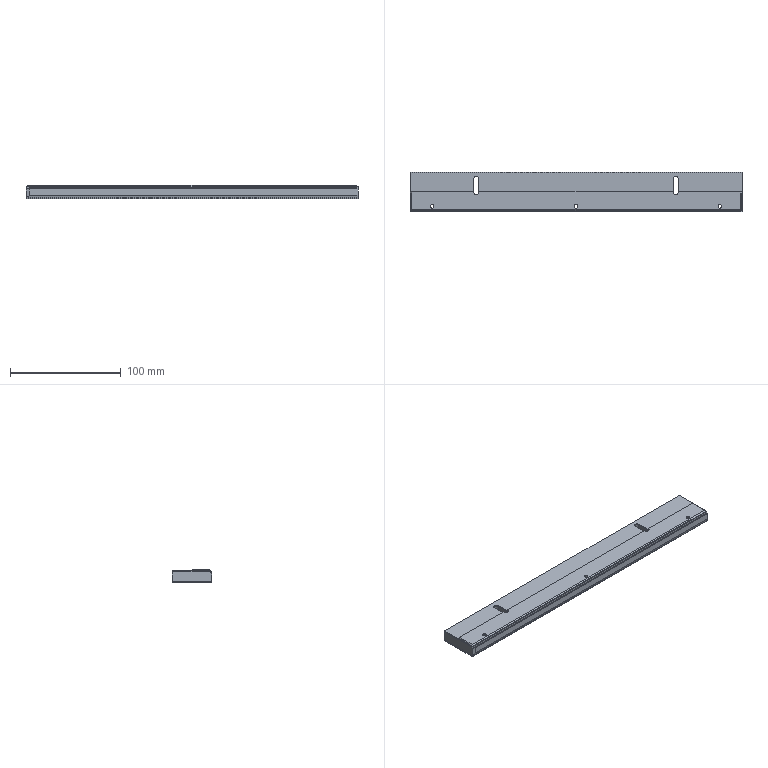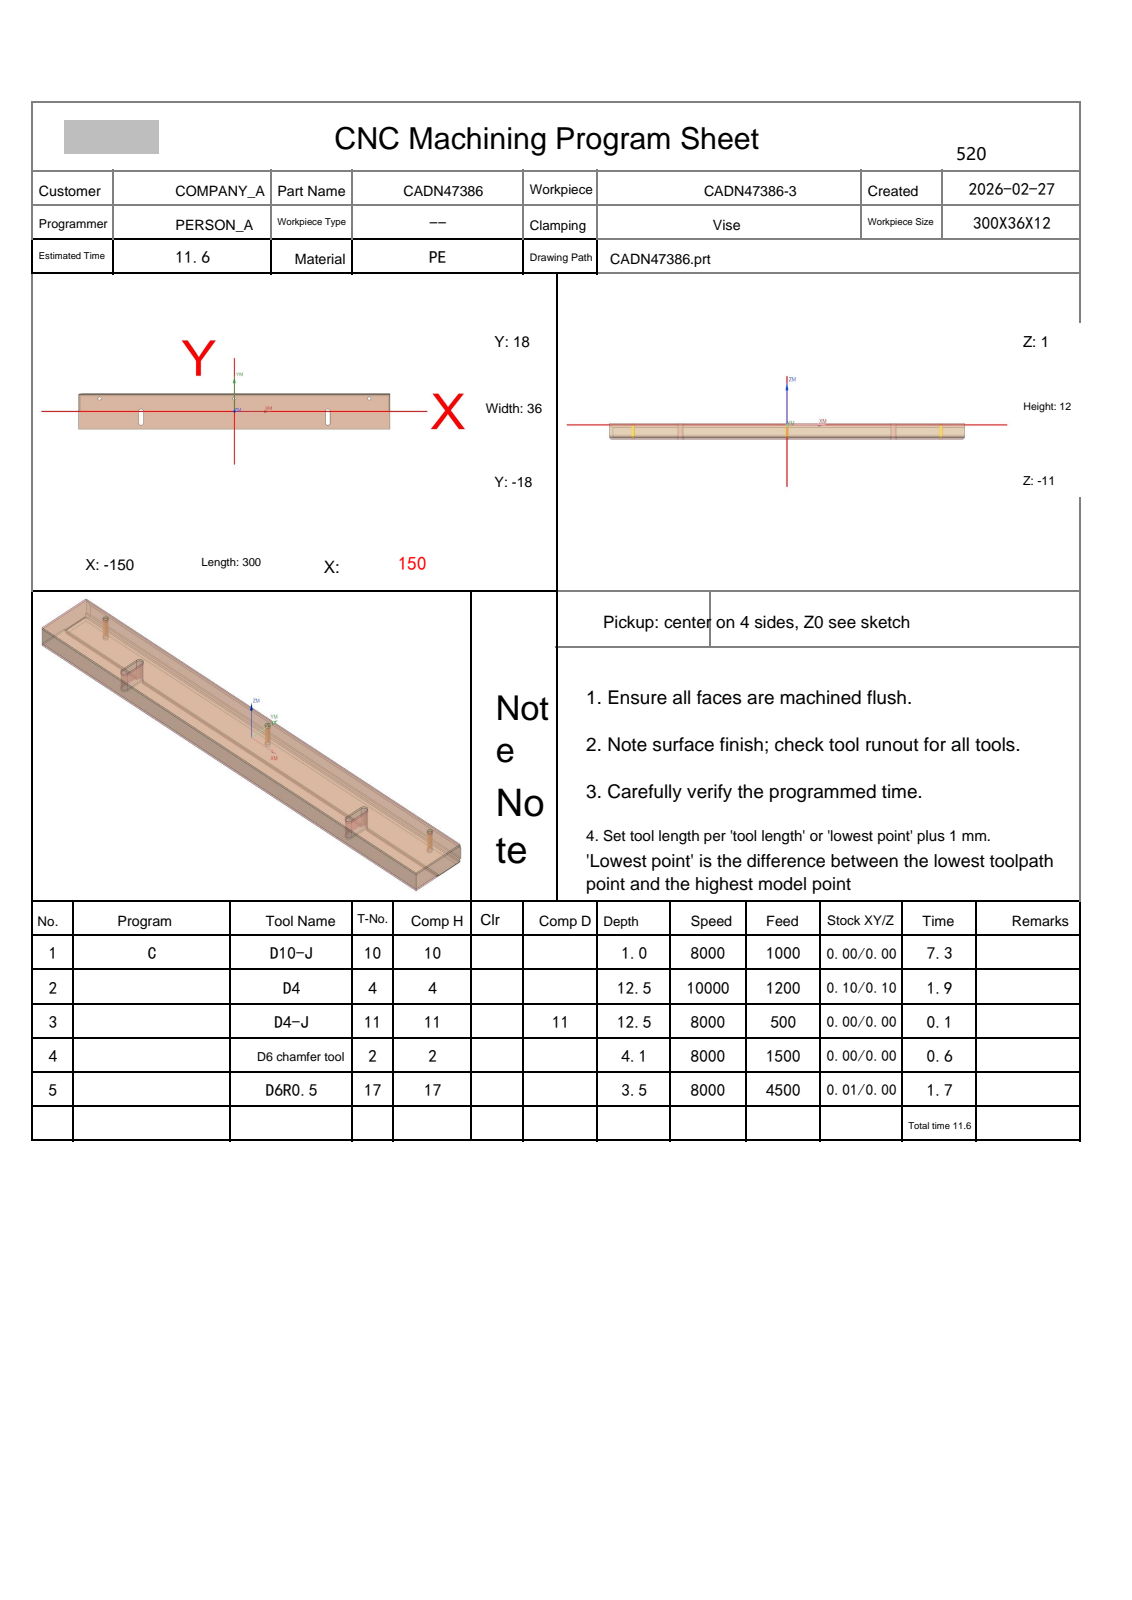NC program | NX | posted by the shop | part box 300 x 36 x 12 mm
Whole program:
%
O0001
(Machine time: 12.95 MIN)
(===Total Tool:5===)
(T10=D10-J  D=10.  R=0.   D-  H10 Z=-0.   )
(T4=D4      D=4.   R=0.   D-  H04 Z=-10.5 )
(T11=D4-J   D=4.   R=0.   D11 H11 Z=-10.5 )
(T2=D6 chamfer tool   D=6.   R=0.   D-  H02 Z=-2.15 )
(T17=D6R0.5 D=6.   R=0.5  D-  H17 Z=-2.5  )
G80 G90 G17 G49 G40
G91 G28 Z0
M01
N1 T10 M06
(D10-J  D=10. R=0. H=10 ce=0.00 di=0.10)
G00 G90 G54 X-167. Y1.111 M03 S8000
G43 H10 Z50.
M08
Z2.55
G01 Z.55 F1000.
X-155. Y13.111
X-145.111 Y23.
X-135.222
X-155. Y3.222
Y-6.667
X-125.333 Y23.
X-115.444
X-155. Y-16.556
Y-23.
X-151.556
X-105.556 Y23.
X-95.667
X-141.667 Y-23.
X-131.778
X-85.778 Y23.
X-75.889
X-121.889 Y-23.
X-112.
X-66. Y23.
X-56.111
X-102.111 Y-23.
X-92.222
X-46.222 Y23.
X-36.333
X-82.333 Y-23.
X-72.444
X-26.444 Y23.
X-16.556
X-62.556 Y-23.
X-52.667
X-6.667 Y23.
X3.222
X-42.778 Y-23.
X-32.889
X13.111 Y23.
X23.
X-23. Y-23.
X-13.111
X32.889 Y23.
X42.778
X-3.222 Y-23.
X6.667
X52.667 Y23.
X62.556
X16.556 Y-23.
X26.444
X72.444 Y23.
X82.333
X36.333 Y-23.
X46.222
X92.222 Y23.
X102.111
X56.111 Y-23.
X66.
X112. Y23.
X121.889
X75.889 Y-23.
X85.778
X131.778 Y23.
X141.667
X95.667 Y-23.
X105.556
X151.556 Y23.
X155.
Y16.556
X115.444 Y-23.
X125.333
X155. Y6.667
Y-3.222
X135.222 Y-23.
X145.111
X155. Y-13.111
X167. Y-1.111
Z2.55
G00 Z4.
X-167. Y1.111
Z2.1
G01 Z.1
X-155. Y13.111
X-145.111 Y23.
X-135.222
X-155. Y3.222
Y-6.667
X-125.333 Y23.
X-115.444
X-155. Y-16.556
Y-23.
X-151.556
X-105.556 Y23.
X-95.667
X-141.667 Y-23.
X-131.778
X-85.778 Y23.
X-75.889
X-121.889 Y-23.
X-112.
X-66. Y23.
X-56.111
X-102.111 Y-23.
X-92.222
X-46.222 Y23.
X-36.333
X-82.333 Y-23.
X-72.444
X-26.444 Y23.
X-16.556
X-62.556 Y-23.
X-52.667
X-6.667 Y23.
X3.222
X-42.778 Y-23.
X-32.889
X13.111 Y23.
X23.
X-23. Y-23.
X-13.111
X32.889 Y23.
X42.778
X-3.222 Y-23.
X6.667
X52.667 Y23.
X62.556
X16.556 Y-23.
X26.444
X72.444 Y23.
X82.333
X36.333 Y-23.
X46.222
X92.222 Y23.
X102.111
X56.111 Y-23.
X66.
X112. Y23.
X121.889
X75.889 Y-23.
X85.778
X131.778 Y23.
X141.667
X95.667 Y-23.
X105.556
X151.556 Y23.
X155.
Y16.556
X115.444 Y-23.
X125.333
X155. Y6.667
Y-3.222
X135.222 Y-23.
X145.111
X155. Y-13.111
X167. Y-1.111
Z2.1
G00 Z50.
G00 G90 X-167. Y1.111 M03 S8000
Z50.
Z2.
G01 Z0.0 F1000.
X-155. Y13.111
X-145.111 Y23.
X-135.222
X-155. Y3.222
Y-6.667
X-125.333 Y23.
X-115.444
X-155. Y-16.556
Y-23.
X-151.556
X-105.556 Y23.
X-95.667
X-141.667 Y-23.
X-131.778
X-85.778 Y23.
X-75.889
X-121.889 Y-23.
X-112.
X-66. Y23.
X-56.111
X-102.111 Y-23.
X-92.222
X-46.222 Y23.
X-36.333
X-82.333 Y-23.
X-72.444
X-26.444 Y23.
X-16.556
X-62.556 Y-23.
X-52.667
X-6.667 Y23.
X3.222
X-42.778 Y-23.
X-32.889
X13.111 Y23.
X23.
X-23. Y-23.
X-13.111
X32.889 Y23.
X42.778
X-3.222 Y-23.
X6.667
X52.667 Y23.
X62.556
X16.556 Y-23.
X26.444
X72.444 Y23.
X82.333
X36.333 Y-23.
X46.222
X92.222 Y23.
X102.111
X56.111 Y-23.
X66.
X112. Y23.
X121.889
X75.889 Y-23.
X85.778
X131.778 Y23.
X141.667
X95.667 Y-23.
X105.556
X151.556 Y23.
X155.
Y16.556
X115.444 Y-23.
X125.333
X155. Y6.667
Y-3.222
X135.222 Y-23.
X145.111
X155. Y-13.111
X167. Y-1.111
Z2.
G00 Z50.
G91 G28 Z0.0
M05
M09
G91 G28 Z0.0
M01
N2 T04 M06
(D4  D=4. R=0. H=04 ce=0.10 di=0.10)
G00 G90 G54 X89.85 Y-5.8 M03 S10000
G43 H04 Z50.
M08
Z.5
G01 Y-11.8 Z.44 F1200.
G03 X90. Y-11.95 Z.438 I.15 J0.0
X90.15 Y-11.8 Z.435 I0.0 J.15
G01 Y.2 Z.315
G03 X90. Y.35 Z.313 I-.15 J0.0
X89.85 Y.2 Z.31 I0.0 J-.15
G01 Y-11.8 Z.19
G03 X90. Y-11.95 Z.188 I.15 J0.0
X90.15 Y-11.8 Z.185 I0.0 J.15
G01 Y.2 Z.065
G03 X90. Y.35 Z.063 I-.15 J0.0
X89.85 Y.2 Z.06 I0.0 J-.15
G01 Y-11.8 Z-.06
G03 X90. Y-11.95 Z-.063 I.15 J0.0
X90.15 Y-11.8 Z-.065 I0.0 J.15
G01 Y.2 Z-.185
G03 X90. Y.35 Z-.188 I-.15 J0.0
X89.85 Y.2 Z-.19 I0.0 J-.15
G01 Y-11.8 Z-.31
G03 X90. Y-11.95 Z-.313 I.15 J0.0
X90.15 Y-11.8 Z-.315 I0.0 J.15
G01 Y.2 Z-.435
G03 X90. Y.35 Z-.438 I-.15 J0.0
X89.85 Y.2 Z-.44 I0.0 J-.15
G01 Y-11.8 Z-.56
G03 X90. Y-11.95 Z-.563 I.15 J0.0
X90.15 Y-11.8 Z-.565 I0.0 J.15
G01 Y.2 Z-.685
G03 X90. Y.35 Z-.688 I-.15 J0.0
X89.85 Y.2 Z-.69 I0.0 J-.15
G01 Y-11.8 Z-.81
G03 X90. Y-11.95 Z-.813 I.15 J0.0
X90.15 Y-11.8 Z-.815 I0.0 J.15
G01 Y.2 Z-.935
G03 X90. Y.35 Z-.938 I-.15 J0.0
X89.85 Y.2 Z-.94 I0.0 J-.15
G01 Y-11.8 Z-1.06
G03 X90. Y-11.95 Z-1.063 I.15 J0.0
X90.15 Y-11.8 Z-1.065 I0.0 J.15
G01 Y.2 Z-1.185
G03 X90. Y.35 Z-1.188 I-.15 J0.0
X89.85 Y.2 Z-1.19 I0.0 J-.15
G01 Y-11.8 Z-1.31
G03 X90. Y-11.95 Z-1.313 I.15 J0.0
X90.15 Y-11.8 Z-1.315 I0.0 J.15
G01 Y.2 Z-1.435
G03 X90. Y.35 Z-1.438 I-.15 J0.0
X89.85 Y.2 Z-1.44 I0.0 J-.15
G01 Y-11.8 Z-1.56
G03 X90. Y-11.95 Z-1.563 I.15 J0.0
X90.15 Y-11.8 Z-1.565 I0.0 J.15
G01 Y.2 Z-1.685
G03 X90. Y.35 Z-1.688 I-.15 J0.0
X89.85 Y.2 Z-1.69 I0.0 J-.15
G01 Y-11.8 Z-1.81
G03 X90. Y-11.95 Z-1.813 I.15 J0.0
X90.15 Y-11.8 Z-1.815 I0.0 J.15
G01 Y.2 Z-1.935
G03 X90. Y.35 Z-1.938 I-.15 J0.0
X89.85 Y.2 Z-1.94 I0.0 J-.15
G01 Y-11.8 Z-2.06
G03 X90. Y-11.95 Z-2.063 I.15 J0.0
X90.15 Y-11.8 Z-2.065 I0.0 J.15
G01 Y.2 Z-2.185
G03 X90. Y.35 Z-2.188 I-.15 J0.0
X89.85 Y.2 Z-2.19 I0.0 J-.15
G01 Y-11.8 Z-2.31
G03 X90. Y-11.95 Z-2.313 I.15 J0.0
X90.15 Y-11.8 Z-2.315 I0.0 J.15
G01 Y.2 Z-2.435
G03 X90. Y.35 Z-2.438 I-.15 J0.0
X89.85 Y.2 Z-2.44 I0.0 J-.15
G01 Y-11.8 Z-2.56
G03 X90. Y-11.95 Z-2.563 I.15 J0.0
X90.15 Y-11.8 Z-2.565 I0.0 J.15
G01 Y.2 Z-2.685
G03 X90. Y.35 Z-2.688 I-.15 J0.0
X89.85 Y.2 Z-2.69 I0.0 J-.15
G01 Y-11.8 Z-2.81
G03 X90. Y-11.95 Z-2.813 I.15 J0.0
X90.15 Y-11.8 Z-2.815 I0.0 J.15
G01 Y.2 Z-2.935
G03 X90. Y.35 Z-2.938 I-.15 J0.0
X89.85 Y.2 Z-2.94 I0.0 J-.15
G01 Y-11.8 Z-3.06
G03 X90. Y-11.95 Z-3.063 I.15 J0.0
X90.15 Y-11.8 Z-3.065 I0.0 J.15
G01 Y.2 Z-3.185
G03 X90. Y.35 Z-3.188 I-.15 J0.0
X89.85 Y.2 Z-3.19 I0.0 J-.15
G01 Y-11.8 Z-3.31
G03 X90. Y-11.95 Z-3.313 I.15 J0.0
X90.15 Y-11.8 Z-3.315 I0.0 J.15
G01 Y.2 Z-3.435
G03 X90. Y.35 Z-3.438 I-.15 J0.0
X89.85 Y.2 Z-3.44 I0.0 J-.15
G01 Y-11.8 Z-3.56
G03 X90. Y-11.95 Z-3.563 I.15 J0.0
X90.15 Y-11.8 Z-3.565 I0.0 J.15
G01 Y.2 Z-3.685
G03 X90. Y.35 Z-3.688 I-.15 J0.0
X89.85 Y.2 Z-3.69 I0.0 J-.15
G01 Y-11.8 Z-3.81
G03 X90. Y-11.95 Z-3.813 I.15 J0.0
X90.15 Y-11.8 Z-3.815 I0.0 J.15
G01 Y.2 Z-3.935
G03 X90. Y.35 Z-3.938 I-.15 J0.0
X89.85 Y.2 Z-3.94 I0.0 J-.15
G01 Y-11.8 Z-4.06
G03 X90. Y-11.95 Z-4.063 I.15 J0.0
X90.15 Y-11.8 Z-4.065 I0.0 J.15
G01 Y.2 Z-4.185
G03 X90. Y.35 Z-4.188 I-.15 J0.0
X89.85 Y.2 Z-4.19 I0.0 J-.15
G01 Y-11.8 Z-4.31
G03 X90. Y-11.95 Z-4.313 I.15 J0.0
X90.15 Y-11.8 Z-4.315 I0.0 J.15
G01 Y.2 Z-4.435
G03 X90. Y.35 Z-4.438 I-.15 J0.0
X89.85 Y.2 Z-4.44 I0.0 J-.15
G01 Y-11.8 Z-4.56
G03 X90. Y-11.95 Z-4.563 I.15 J0.0
X90.15 Y-11.8 Z-4.565 I0.0 J.15
G01 Y.2 Z-4.685
G03 X90. Y.35 Z-4.688 I-.15 J0.0
X89.85 Y.2 Z-4.69 I0.0 J-.15
G01 Y-11.8 Z-4.81
G03 X90. Y-11.95 Z-4.813 I.15 J0.0
X90.15 Y-11.8 Z-4.815 I0.0 J.15
G01 Y.2 Z-4.935
G03 X90. Y.35 Z-4.938 I-.15 J0.0
X89.85 Y.2 Z-4.94 I0.0 J-.15
G01 Y-11.8 Z-5.06
G03 X90. Y-11.95 Z-5.063 I.15 J0.0
X90.15 Y-11.8 Z-5.065 I0.0 J.15
G01 Y.2 Z-5.185
G03 X90. Y.35 Z-5.188 I-.15 J0.0
X89.85 Y.2 Z-5.19 I0.0 J-.15
G01 Y-11.8 Z-5.31
G03 X90. Y-11.95 Z-5.313 I.15 J0.0
X90.15 Y-11.8 Z-5.315 I0.0 J.15
G01 Y.2 Z-5.435
G03 X90. Y.35 Z-5.438 I-.15 J0.0
X89.85 Y.2 Z-5.44 I0.0 J-.15
G01 Y-11.8 Z-5.56
G03 X90. Y-11.95 Z-5.563 I.15 J0.0
X90.15 Y-11.8 Z-5.565 I0.0 J.15
G01 Y.2 Z-5.685
G03 X90. Y.35 Z-5.688 I-.15 J0.0
X89.85 Y.2 Z-5.69 I0.0 J-.15
G01 Y-11.8 Z-5.81
G03 X90. Y-11.95 Z-5.813 I.15 J0.0
X90.15 Y-11.8 Z-5.815 I0.0 J.15
G01 Y.2 Z-5.935
G03 X90. Y.35 Z-5.938 I-.15 J0.0
X89.85 Y.2 Z-5.94 I0.0 J-.15
G01 Y-11.8 Z-6.06
G03 X90. Y-11.95 Z-6.063 I.15 J0.0
X90.15 Y-11.8 Z-6.065 I0.0 J.15
G01 Y.2 Z-6.185
G03 X90. Y.35 Z-6.188 I-.15 J0.0
X89.85 Y.2 Z-6.19 I0.0 J-.15
G01 Y-11.8 Z-6.31
G03 X90. Y-11.95 Z-6.313 I.15 J0.0
X90.15 Y-11.8 Z-6.315 I0.0 J.15
G01 Y.2 Z-6.435
G03 X90. Y.35 Z-6.438 I-.15 J0.0
X89.85 Y.2 Z-6.44 I0.0 J-.15
G01 Y-11.8 Z-6.56
G03 X90. Y-11.95 Z-6.563 I.15 J0.0
X90.15 Y-11.8 Z-6.565 I0.0 J.15
G01 Y.2 Z-6.685
G03 X90. Y.35 Z-6.688 I-.15 J0.0
X89.85 Y.2 Z-6.69 I0.0 J-.15
G01 Y-11.8 Z-6.81
G03 X90. Y-11.95 Z-6.813 I.15 J0.0
X90.15 Y-11.8 Z-6.815 I0.0 J.15
G01 Y.2 Z-6.935
G03 X90. Y.35 Z-6.938 I-.15 J0.0
X89.85 Y.2 Z-6.94 I0.0 J-.15
G01 Y-11.8 Z-7.06
G03 X90. Y-11.95 Z-7.063 I.15 J0.0
X90.15 Y-11.8 Z-7.065 I0.0 J.15
G01 Y.2 Z-7.185
G03 X90. Y.35 Z-7.188 I-.15 J0.0
X89.85 Y.2 Z-7.19 I0.0 J-.15
G01 Y-11.8 Z-7.31
G03 X90. Y-11.95 Z-7.313 I.15 J0.0
X90.15 Y-11.8 Z-7.315 I0.0 J.15
G01 Y.2 Z-7.435
G03 X90. Y.35 Z-7.438 I-.15 J0.0
X89.85 Y.2 Z-7.44 I0.0 J-.15
G01 Y-11.8 Z-7.56
G03 X90. Y-11.95 Z-7.563 I.15 J0.0
X90.15 Y-11.8 Z-7.565 I0.0 J.15
G01 Y.2 Z-7.685
G03 X90. Y.35 Z-7.688 I-.15 J0.0
X89.85 Y.2 Z-7.69 I0.0 J-.15
G01 Y-11.8 Z-7.81
G03 X90. Y-11.95 Z-7.813 I.15 J0.0
X90.15 Y-11.8 Z-7.815 I0.0 J.15
G01 Y.2 Z-7.935
G03 X90. Y.35 Z-7.938 I-.15 J0.0
X89.85 Y.2 Z-7.94 I0.0 J-.15
G01 Y-11.8 Z-8.06
G03 X90. Y-11.95 Z-8.063 I.15 J0.0
X90.15 Y-11.8 Z-8.065 I0.0 J.15
G01 Y.2 Z-8.185
G03 X90. Y.35 Z-8.188 I-.15 J0.0
X89.85 Y.2 Z-8.19 I0.0 J-.15
G01 Y-11.8 Z-8.31
G03 X90. Y-11.95 Z-8.313 I.15 J0.0
X90.15 Y-11.8 Z-8.315 I0.0 J.15
G01 Y.2 Z-8.435
G03 X90. Y.35 Z-8.438 I-.15 J0.0
X89.85 Y.2 Z-8.44 I0.0 J-.15
G01 Y-11.8 Z-8.56
G03 X90. Y-11.95 Z-8.563 I.15 J0.0
X90.15 Y-11.8 Z-8.565 I0.0 J.15
G01 Y.2 Z-8.685
G03 X90. Y.35 Z-8.688 I-.15 J0.0
X89.85 Y.2 Z-8.69 I0.0 J-.15
G01 Y-11.8 Z-8.81
G03 X90. Y-11.95 Z-8.813 I.15 J0.0
X90.15 Y-11.8 Z-8.815 I0.0 J.15
G01 Y.2 Z-8.935
G03 X90. Y.35 Z-8.938 I-.15 J0.0
X89.85 Y.2 Z-8.94 I0.0 J-.15
G01 Y-11.8 Z-9.06
G03 X90. Y-11.95 Z-9.063 I.15 J0.0
X90.15 Y-11.8 Z-9.065 I0.0 J.15
G01 Y.2 Z-9.185
G03 X90. Y.35 Z-9.188 I-.15 J0.0
X89.85 Y.2 Z-9.19 I0.0 J-.15
G01 Y-11.8 Z-9.31
G03 X90. Y-11.95 Z-9.313 I.15 J0.0
X90.15 Y-11.8 Z-9.315 I0.0 J.15
G01 Y.2 Z-9.435
G03 X90. Y.35 Z-9.438 I-.15 J0.0
X89.85 Y.2 Z-9.44 I0.0 J-.15
G01 Y-11.8 Z-9.56
G03 X90. Y-11.95 Z-9.563 I.15 J0.0
X90.15 Y-11.8 Z-9.565 I0.0 J.15
G01 Y.2 Z-9.685
G03 X90. Y.35 Z-9.688 I-.15 J0.0
X89.85 Y.2 Z-9.69 I0.0 J-.15
G01 Y-11.8 Z-9.81
G03 X90. Y-11.95 Z-9.813 I.15 J0.0
X90.15 Y-11.8 Z-9.815 I0.0 J.15
G01 Y.2 Z-9.935
G03 X90. Y.35 Z-9.938 I-.15 J0.0
X89.85 Y.2 Z-9.94 I0.0 J-.15
G01 Y-11.8 Z-10.06
G03 X90. Y-11.95 Z-10.063 I.15 J0.0
X90.15 Y-11.8 Z-10.065 I0.0 J.15
G01 Y.2 Z-10.185
G03 X90. Y.35 Z-10.188 I-.15 J0.0
X89.85 Y.2 Z-10.19 I0.0 J-.15
G01 Y-11.8 Z-10.31
G03 X90. Y-11.95 Z-10.313 I.15 J0.0
X90.15 Y-11.8 Z-10.315 I0.0 J.15
G01 Y.2 Z-10.435
G03 X90. Y.35 Z-10.438 I-.15 J0.0
X89.85 Y.2 Z-10.44 I0.0 J-.15
G01 Y-5.8 Z-10.5
Y-11.8
G03 X90. Y-11.95 I.15 J0.0
X90.15 Y-11.8 I0.0 J.15
G01 Y.2
G03 X90. Y.35 I-.15 J0.0
X89.85 Y.2 I0.0 J-.15
G01 Y-5.8
Y-6.3
Z-9.5
G00 Z50.
X-89.85 Y-5.8
Z.5
G01 Y.2 Z.44
G03 X-90. Y.35 Z.438 I-.15 J0.0
X-90.15 Y.2 Z.435 I0.0 J-.15
G01 Y-11.8 Z.315
G03 X-90. Y-11.95 Z.313 I.15 J0.0
X-89.85 Y-11.8 Z.31 I0.0 J.15
G01 Y.2 Z.19
G03 X-90. Y.35 Z.188 I-.15 J0.0
X-90.15 Y.2 Z.185 I0.0 J-.15
G01 Y-11.8 Z.065
G03 X-90. Y-11.95 Z.063 I.15 J0.0
X-89.85 Y-11.8 Z.06 I0.0 J.15
G01 Y.2 Z-.06
G03 X-90. Y.35 Z-.063 I-.15 J0.0
X-90.15 Y.2 Z-.065 I0.0 J-.15
G01 Y-11.8 Z-.185
G03 X-90. Y-11.95 Z-.188 I.15 J0.0
X-89.85 Y-11.8 Z-.19 I0.0 J.15
G01 Y.2 Z-.31
G03 X-90. Y.35 Z-.313 I-.15 J0.0
X-90.15 Y.2 Z-.315 I0.0 J-.15
G01 Y-11.8 Z-.435
G03 X-90. Y-11.95 Z-.438 I.15 J0.0
X-89.85 Y-11.8 Z-.44 I0.0 J.15
G01 Y.2 Z-.56
G03 X-90. Y.35 Z-.563 I-.15 J0.0
X-90.15 Y.2 Z-.565 I0.0 J-.15
G01 Y-11.8 Z-.685
G03 X-90. Y-11.95 Z-.688 I.15 J0.0
X-89.85 Y-11.8 Z-.69 I0.0 J.15
G01 Y.2 Z-.81
G03 X-90. Y.35 Z-.813 I-.15 J0.0
X-90.15 Y.2 Z-.815 I0.0 J-.15
G01 Y-11.8 Z-.935
G03 X-90. Y-11.95 Z-.938 I.15 J0.0
X-89.85 Y-11.8 Z-.94 I0.0 J.15
G01 Y.2 Z-1.06
G03 X-90. Y.35 Z-1.063 I-.15 J0.0
X-90.15 Y.2 Z-1.065 I0.0 J-.15
G01 Y-11.8 Z-1.185
G03 X-90. Y-11.95 Z-1.188 I.15 J0.0
X-89.85 Y-11.8 Z-1.19 I0.0 J.15
G01 Y.2 Z-1.31
G03 X-90. Y.35 Z-1.313 I-.15 J0.0
X-90.15 Y.2 Z-1.315 I0.0 J-.15
G01 Y-11.8 Z-1.435
G03 X-90. Y-11.95 Z-1.438 I.15 J0.0
X-89.85 Y-11.8 Z-1.44 I0.0 J.15
G01 Y.2 Z-1.56
G03 X-90. Y.35 Z-1.563 I-.15 J0.0
X-90.15 Y.2 Z-1.565 I0.0 J-.15
G01 Y-11.8 Z-1.685
G03 X-90. Y-11.95 Z-1.688 I.15 J0.0
X-89.85 Y-11.8 Z-1.69 I0.0 J.15
G01 Y.2 Z-1.81
G03 X-90. Y.35 Z-1.813 I-.15 J0.0
X-90.15 Y.2 Z-1.815 I0.0 J-.15
G01 Y-11.8 Z-1.935
G03 X-90. Y-11.95 Z-1.938 I.15 J0.0
X-89.85 Y-11.8 Z-1.94 I0.0 J.15
G01 Y.2 Z-2.06
G03 X-90. Y.35 Z-2.063 I-.15 J0.0
X-90.15 Y.2 Z-2.065 I0.0 J-.15
G01 Y-11.8 Z-2.185
G03 X-90. Y-11.95 Z-2.188 I.15 J0.0
X-89.85 Y-11.8 Z-2.19 I0.0 J.15
G01 Y.2 Z-2.31
G03 X-90. Y.35 Z-2.313 I-.15 J0.0
X-90.15 Y.2 Z-2.315 I0.0 J-.15
G01 Y-11.8 Z-2.435
G03 X-90. Y-11.95 Z-2.438 I.15 J0.0
X-89.85 Y-11.8 Z-2.44 I0.0 J.15
G01 Y.2 Z-2.56
G03 X-90. Y.35 Z-2.563 I-.15 J0.0
X-90.15 Y.2 Z-2.565 I0.0 J-.15
G01 Y-11.8 Z-2.685
G03 X-90. Y-11.95 Z-2.688 I.15 J0.0
X-89.85 Y-11.8 Z-2.69 I0.0 J.15
G01 Y.2 Z-2.81
G03 X-90. Y.35 Z-2.813 I-.15 J0.0
X-90.15 Y.2 Z-2.815 I0.0 J-.15
G01 Y-11.8 Z-2.935
G03 X-90. Y-11.95 Z-2.938 I.15 J0.0
X-89.85 Y-11.8 Z-2.94 I0.0 J.15
G01 Y.2 Z-3.06
G03 X-90. Y.35 Z-3.063 I-.15 J0.0
X-90.15 Y.2 Z-3.065 I0.0 J-.15
G01 Y-11.8 Z-3.185
G03 X-90. Y-11.95 Z-3.188 I.15 J0.0
X-89.85 Y-11.8 Z-3.19 I0.0 J.15
G01 Y.2 Z-3.31
G03 X-90. Y.35 Z-3.313 I-.15 J0.0
X-90.15 Y.2 Z-3.315 I0.0 J-.15
G01 Y-11.8 Z-3.435
G03 X-90. Y-11.95 Z-3.438 I.15 J0.0
X-89.85 Y-11.8 Z-3.44 I0.0 J.15
G01 Y.2 Z-3.56
G03 X-90. Y.35 Z-3.563 I-.15 J0.0
X-90.15 Y.2 Z-3.565 I0.0 J-.15
G01 Y-11.8 Z-3.685
G03 X-90. Y-11.95 Z-3.688 I.15 J0.0
X-89.85 Y-11.8 Z-3.69 I0.0 J.15
G01 Y.2 Z-3.81
G03 X-90. Y.35 Z-3.813 I-.15 J0.0
X-90.15 Y.2 Z-3.815 I0.0 J-.15
G01 Y-11.8 Z-3.935
G03 X-90. Y-11.95 Z-3.938 I.15 J0.0
X-89.85 Y-11.8 Z-3.94 I0.0 J.15
G01 Y.2 Z-4.06
G03 X-90. Y.35 Z-4.063 I-.15 J0.0
X-90.15 Y.2 Z-4.065 I0.0 J-.15
G01 Y-11.8 Z-4.185
G03 X-90. Y-11.95 Z-4.188 I.15 J0.0
X-89.85 Y-11.8 Z-4.19 I0.0 J.15
G01 Y.2 Z-4.31
G03 X-90. Y.35 Z-4.313 I-.15 J0.0
X-90.15 Y.2 Z-4.315 I0.0 J-.15
G01 Y-11.8 Z-4.435
G03 X-90. Y-11.95 Z-4.438 I.15 J0.0
X-89.85 Y-11.8 Z-4.44 I0.0 J.15
G01 Y.2 Z-4.56
G03 X-90. Y.35 Z-4.563 I-.15 J0.0
X-90.15 Y.2 Z-4.565 I0.0 J-.15
G01 Y-11.8 Z-4.685
G03 X-90. Y-11.95 Z-4.688 I.15 J0.0
X-89.85 Y-11.8 Z-4.69 I0.0 J.15
G01 Y.2 Z-4.81
G03 X-90. Y.35 Z-4.813 I-.15 J0.0
X-90.15 Y.2 Z-4.815 I0.0 J-.15
G01 Y-11.8 Z-4.935
G03 X-90. Y-11.95 Z-4.938 I.15 J0.0
X-89.85 Y-11.8 Z-4.94 I0.0 J.15
G01 Y.2 Z-5.06
G03 X-90. Y.35 Z-5.063 I-.15 J0.0
X-90.15 Y.2 Z-5.065 I0.0 J-.15
G01 Y-11.8 Z-5.185
G03 X-90. Y-11.95 Z-5.188 I.15 J0.0
X-89.85 Y-11.8 Z-5.19 I0.0 J.15
G01 Y.2 Z-5.31
G03 X-90. Y.35 Z-5.313 I-.15 J0.0
X-90.15 Y.2 Z-5.315 I0.0 J-.15
G01 Y-11.8 Z-5.435
G03 X-90. Y-11.95 Z-5.438 I.15 J0.0
X-89.85 Y-11.8 Z-5.44 I0.0 J.15
G01 Y.2 Z-5.56
G03 X-90. Y.35 Z-5.563 I-.15 J0.0
X-90.15 Y.2 Z-5.565 I0.0 J-.15
G01 Y-11.8 Z-5.685
G03 X-90. Y-11.95 Z-5.688 I.15 J0.0
X-89.85 Y-11.8 Z-5.69 I0.0 J.15
G01 Y.2 Z-5.81
G03 X-90. Y.35 Z-5.813 I-.15 J0.0
X-90.15 Y.2 Z-5.815 I0.0 J-.15
G01 Y-11.8 Z-5.935
G03 X-90. Y-11.95 Z-5.938 I.15 J0.0
X-89.85 Y-11.8 Z-5.94 I0.0 J.15
G01 Y.2 Z-6.06
G03 X-90. Y.35 Z-6.063 I-.15 J0.0
X-90.15 Y.2 Z-6.065 I0.0 J-.15
G01 Y-11.8 Z-6.185
G03 X-90. Y-11.95 Z-6.188 I.15 J0.0
X-89.85 Y-11.8 Z-6.19 I0.0 J.15
G01 Y.2 Z-6.31
G03 X-90. Y.35 Z-6.313 I-.15 J0.0
X-90.15 Y.2 Z-6.315 I0.0 J-.15
G01 Y-11.8 Z-6.435
G03 X-90. Y-11.95 Z-6.438 I.15 J0.0
X-89.85 Y-11.8 Z-6.44 I0.0 J.15
G01 Y.2 Z-6.56
G03 X-90. Y.35 Z-6.563 I-.15 J0.0
X-90.15 Y.2 Z-6.565 I0.0 J-.15
G01 Y-11.8 Z-6.685
G03 X-90. Y-11.95 Z-6.688 I.15 J0.0
X-89.85 Y-11.8 Z-6.69 I0.0 J.15
G01 Y.2 Z-6.81
G03 X-90. Y.35 Z-6.813 I-.15 J0.0
X-90.15 Y.2 Z-6.815 I0.0 J-.15
G01 Y-11.8 Z-6.935
G03 X-90. Y-11.95 Z-6.938 I.15 J0.0
X-89.85 Y-11.8 Z-6.94 I0.0 J.15
G01 Y.2 Z-7.06
G03 X-90. Y.35 Z-7.063 I-.15 J0.0
X-90.15 Y.2 Z-7.065 I0.0 J-.15
G01 Y-11.8 Z-7.185
G03 X-90. Y-11.95 Z-7.188 I.15 J0.0
X-89.85 Y-11.8 Z-7.19 I0.0 J.15
G01 Y.2 Z-7.31
G03 X-90. Y.35 Z-7.313 I-.15 J0.0
X-90.15 Y.2 Z-7.315 I0.0 J-.15
G01 Y-11.8 Z-7.435
G03 X-90. Y-11.95 Z-7.438 I.15 J0.0
X-89.85 Y-11.8 Z-7.44 I0.0 J.15
G01 Y.2 Z-7.56
G03 X-90. Y.35 Z-7.563 I-.15 J0.0
X-90.15 Y.2 Z-7.565 I0.0 J-.15
G01 Y-11.8 Z-7.685
G03 X-90. Y-11.95 Z-7.688 I.15 J0.0
X-89.85 Y-11.8 Z-7.69 I0.0 J.15
G01 Y.2 Z-7.81
G03 X-90. Y.35 Z-7.813 I-.15 J0.0
X-90.15 Y.2 Z-7.815 I0.0 J-.15
G01 Y-11.8 Z-7.935
G03 X-90. Y-11.95 Z-7.938 I.15 J0.0
X-89.85 Y-11.8 Z-7.94 I0.0 J.15
G01 Y.2 Z-8.06
G03 X-90. Y.35 Z-8.063 I-.15 J0.0
X-90.15 Y.2 Z-8.065 I0.0 J-.15
G01 Y-11.8 Z-8.185
G03 X-90. Y-11.95 Z-8.188 I.15 J0.0
X-89.85 Y-11.8 Z-8.19 I0.0 J.15
G01 Y.2 Z-8.31
G03 X-90. Y.35 Z-8.313 I-.15 J0.0
X-90.15 Y.2 Z-8.315 I0.0 J-.15
G01 Y-11.8 Z-8.435
G03 X-90. Y-11.95 Z-8.438 I.15 J0.0
X-89.85 Y-11.8 Z-8.44 I0.0 J.15
G01 Y.2 Z-8.56
G03 X-90. Y.35 Z-8.563 I-.15 J0.0
X-90.15 Y.2 Z-8.565 I0.0 J-.15
G01 Y-11.8 Z-8.685
G03 X-90. Y-11.95 Z-8.688 I.15 J0.0
X-89.85 Y-11.8 Z-8.69 I0.0 J.15
G01 Y.2 Z-8.81
G03 X-90. Y.35 Z-8.813 I-.15 J0.0
X-90.15 Y.2 Z-8.815 I0.0 J-.15
G01 Y-11.8 Z-8.935
G03 X-90. Y-11.95 Z-8.938 I.15 J0.0
X-89.85 Y-11.8 Z-8.94 I0.0 J.15
G01 Y.2 Z-9.06
G03 X-90. Y.35 Z-9.063 I-.15 J0.0
X-90.15 Y.2 Z-9.065 I0.0 J-.15
G01 Y-11.8 Z-9.185
G03 X-90. Y-11.95 Z-9.188 I.15 J0.0
X-89.85 Y-11.8 Z-9.19 I0.0 J.15
G01 Y.2 Z-9.31
G03 X-90. Y.35 Z-9.313 I-.15 J0.0
X-90.15 Y.2 Z-9.315 I0.0 J-.15
G01 Y-11.8 Z-9.435
G03 X-90. Y-11.95 Z-9.438 I.15 J0.0
X-89.85 Y-11.8 Z-9.44 I0.0 J.15
G01 Y.2 Z-9.56
G03 X-90. Y.35 Z-9.563 I-.15 J0.0
X-90.15 Y.2 Z-9.565 I0.0 J-.15
G01 Y-11.8 Z-9.685
G03 X-90. Y-11.95 Z-9.688 I.15 J0.0
X-89.85 Y-11.8 Z-9.69 I0.0 J.15
G01 Y.2 Z-9.81
G03 X-90. Y.35 Z-9.813 I-.15 J0.0
X-90.15 Y.2 Z-9.815 I0.0 J-.15
G01 Y-11.8 Z-9.935
G03 X-90. Y-11.95 Z-9.938 I.15 J0.0
X-89.85 Y-11.8 Z-9.94 I0.0 J.15
G01 Y.2 Z-10.06
G03 X-90. Y.35 Z-10.063 I-.15 J0.0
X-90.15 Y.2 Z-10.065 I0.0 J-.15
G01 Y-11.8 Z-10.185
G03 X-90. Y-11.95 Z-10.188 I.15 J0.0
X-89.85 Y-11.8 Z-10.19 I0.0 J.15
G01 Y.2 Z-10.31
G03 X-90. Y.35 Z-10.313 I-.15 J0.0
X-90.15 Y.2 Z-10.315 I0.0 J-.15
G01 Y-11.8 Z-10.435
G03 X-90. Y-11.95 Z-10.438 I.15 J0.0
X-89.85 Y-11.8 Z-10.44 I0.0 J.15
G01 Y-5.8 Z-10.5
Y.2
G03 X-90. Y.35 I-.15 J0.0
X-90.15 Y.2 I0.0 J-.15
G01 Y-11.8
G03 X-90. Y-11.95 I.15 J0.0
X-89.85 Y-11.8 I0.0 J.15
G01 Y-5.8
Y-5.3
Z-9.5
G00 Z50.
G91 G28 Z0.0
M05
M09
G91 G28 Z0.0
M01
N3 T11 M06
(D4-J  D=4. R=0. H=11 ce=0.00 di=0.00)
G00 G90 G54 X90. Y-6. M03 S8000
G43 H11 Z50.
M08
Z-3.
G01 Z-3.5 F500.
G41 D11
X90.05
G03 X90.25 Y-5.8 I0.0 J.2
G01 Y.2
G03 X90. Y.45 I-.25 J0.0
X89.75 Y.2 I0.0 J-.25
G01 Y-11.8
G03 X90. Y-12.05 I.25 J0.0
X90.25 Y-11.8 I0.0 J.25
G01 Y-5.8
Y-5.3
G03 X90.05 Y-5.1 I-.2 J0.0
G01 G40 X90.
Z-3.
G00 Z1.
Y-6.
Z-6.5
G01 Z-7.
G41 D11
X90.05
G03 X90.25 Y-5.8 I0.0 J.2
G01 Y.2
G03 X90. Y.45 I-.25 J0.0
X89.75 Y.2 I0.0 J-.25
G01 Y-11.8
G03 X90. Y-12.05 I.25 J0.0
X90.25 Y-11.8 I0.0 J.25
G01 Y-5.8
Y-5.3
G03 X90.05 Y-5.1 I-.2 J0.0
G01 G40 X90.
Z-6.5
G00 Z-2.5
Y-6.
Z-10.
G01 Z-10.5
G41 D11
X90.05
G03 X90.25 Y-5.8 I0.0 J.2
G01 Y.2
G03 X90. Y.45 I-.25 J0.0
X89.75 Y.2 I0.0 J-.25
G01 Y-11.8
G03 X90. Y-12.05 I.25 J0.0
X90.25 Y-11.8 I0.0 J.25
G01 Y-5.8
Y-5.3
G03 X90.05 Y-5.1 I-.2 J0.0
G01 G40 X90.
Z-10.
G00 Z50.
X-90. Y-6.
Z-3.
G01 Z-3.5
G41 D11
X-89.95
G03 X-89.75 Y-5.8 I0.0 J.2
G01 Y.2
G03 X-90. Y.45 I-.25 J0.0
X-90.25 Y.2 I0.0 J-.25
G01 Y-11.8
G03 X-90. Y-12.05 I.25 J0.0
X-89.75 Y-11.8 I0.0 J.25
G01 Y-5.8
Y-5.3
G03 X-89.95 Y-5.1 I-.2 J0.0
G01 G40 X-90.
Z-3.
G00 Z1.
Y-6.
Z-6.5
G01 Z-7.
G41 D11
X-89.95
G03 X-89.75 Y-5.8 I0.0 J.2
G01 Y.2
G03 X-90. Y.45 I-.25 J0.0
X-90.25 Y.2 I0.0 J-.25
G01 Y-11.8
G03 X-90. Y-12.05 I.25 J0.0
X-89.75 Y-11.8 I0.0 J.25
G01 Y-5.8
Y-5.3
G03 X-89.95 Y-5.1 I-.2 J0.0
G01 G40 X-90.
Z-6.5
G00 Z-2.5
Y-6.
Z-10.
G01 Z-10.5
G41 D11
X-89.95
G03 X-89.75 Y-5.8 I0.0 J.2
G01 Y.2
G03 X-90. Y.45 I-.25 J0.0
X-90.25 Y.2 I0.0 J-.25
G01 Y-11.8
G03 X-90. Y-12.05 I.25 J0.0
X-89.75 Y-11.8 I0.0 J.25
G01 Y-5.8
Y-5.3
G03 X-89.95 Y-5.1 I-.2 J0.0
G01 G40 X-90.
Z-10.
G00 Z50.
G91 G28 Z0.0
M05
M09
G91 G28 Z0.0
M01
N4 T02 M06
(D6 chamfer tool  D=6. R=0. H=02 ce=0.00 di=0.00)
G00 G90 G54 X-130. Y13. M03 S8000
G43 H02 Z30.
M08
G98 G81 X-130. Y13. Z-2.15 R3. F500.
X0.0
X130.
G80
G00 Z30.
G00 G90 X-.386 Y18.727 M03 S6500
Z50.
Z.172
G01 Z-1.2 F1500.
G03 X-.1 Y18.527 I1.286 J1.532
G01 X-.054 Y18.497
X0.0 Y18.5
X150.
G02 X151. Y17.5 I0.0 J-1.
G01 Y-18.
G02 X150. Y-19. I-1. J0.0
G01 X-150.
G02 X-151. Y-18. I0.0 J1.
G01 Y17.5
G02 X-150. Y18.5 I1. J0.0
G01 X0.0
X.054 Y18.497
X.1 Y18.527
G03 X.386 Y18.727 I-1. J1.732
G01 Z.172
G00 Z10.
X129.535 Y13.419
Z.413
G01 Z-1.2
G03 X129.388 Y13.103 I1.732 J-1.
G01 X129.367 Y13.053
X129.379 Y13.
G03 X130. Y12.379 I.621 J0.0
X130.621 Y13. I0.0 J.621
X130. Y13.621 I-.621 J0.0
X129.379 Y13. I0.0 J-.621
G01 X129.367 Y12.947
X129.388 Y12.897
G03 X129.535 Y12.581 I1.879 J.684
G01 Z.413
G00 Z10.
X88.977 Y-5.414
Z.172
G01 Z-1.2
G03 X88.777 Y-5.7 I1.532 J-1.286
G01 X88.747 Y-5.746
X88.75 Y-5.8
Y-11.8
G03 X90. Y-13.05 I1.25 J0.0
X91.25 Y-11.8 I0.0 J1.25
G01 Y.2
G03 X90. Y1.45 I-1.25 J0.0
X88.75 Y.2 I0.0 J-1.25
G01 Y-5.8
X88.747 Y-5.854
X88.777 Y-5.9
G03 X88.977 Y-6.186 I1.732 J1.
G01 Z.172
G00 Z10.
X-.465 Y13.419
Z.413
G01 Z-1.2
G03 X-.612 Y13.103 I1.732 J-1.
G01 X-.633 Y13.053
X-.621 Y13.
G03 X0.0 Y12.379 I.621 J0.0
X.621 Y13. I0.0 J.621
X0.0 Y13.621 I-.621 J0.0
X-.621 Y13. I0.0 J-.621
G01 X-.633 Y12.947
X-.612 Y12.897
G03 X-.465 Y12.581 I1.879 J.684
G01 Z.413
G00 Z10.
X-88.977 Y-6.186
Z.172
G01 Z-1.2
G03 X-88.777 Y-5.9 I-1.532 J1.286
G01 X-88.747 Y-5.854
X-88.75 Y-5.8
Y.2
G03 X-90. Y1.45 I-1.25 J0.0
X-91.25 Y.2 I0.0 J-1.25
G01 Y-11.8
G03 X-90. Y-13.05 I1.25 J0.0
X-88.75 Y-11.8 I0.0 J1.25
G01 Y-5.8
X-88.747 Y-5.746
X-88.777 Y-5.7
G03 X-88.977 Y-5.414 I-1.732 J-1.
G01 Z.172
G00 Z10.
X-130.465 Y13.419
Z.413
G01 Z-1.2
G03 X-130.612 Y13.103 I1.732 J-1.
G01 X-130.633 Y13.053
X-130.621 Y13.
G03 X-130. Y12.379 I.621 J0.0
X-129.379 Y13. I0.0 J.621
X-130. Y13.621 I-.621 J0.0
X-130.621 Y13. I0.0 J-.621
G01 X-130.633 Y12.947
X-130.612 Y12.897
G03 X-130.465 Y12.581 I1.879 J.684
G01 Z.413
G00 Z50.
G91 G28 Z0.0
M05
M09
G91 G28 Z0.0
M01
N5 T17 M06
(D6R0.5  D=6. R=0.5 H=17 ce=0.01 di=0.00)
G00 G90 G54 X-156.254 Y20.424 M03 S8000
G43 H17 Z11.077
M08
Z.403
G01 Z-.097 F4500.
X-151.044
X151.07
X151.071 Y20.437 Z-.146
Y20.448 Z-.194
X-151.073
X-151.071 Y20.461 Z-.243
X-151.07 Y20.473 Z-.291
X151.071 Y20.472
Y20.485 Z-.34
Y20.496 Z-.388
X151.051 Y20.497
X-149.316
X-151.067
X-151.066 Y20.51 Z-.437
X-151.064 Y20.521 Z-.485
X-149.316 Y20.522
X151.051
X151.071 Y20.521
Y20.534 Z-.534
Y20.545 Z-.582
X151.051 Y20.546
X-149.316
X-151.061
X-151.06 Y20.558 Z-.631
X-151.058 Y20.57 Z-.679
X-149.316
X151.051
X151.072 Y20.569
Y20.582 Z-.728
Y20.593 Z-.776
X151.051 Y20.594
X-149.316
X-151.055
X-151.054 Y20.607 Z-.825
X-151.052 Y20.619 Z-.873
X-149.258
X151.051
X151.072 Y20.618
Y20.631 Z-.922
Y20.642 Z-.97
X151.051 Y20.643
X-150.704
X-151. Y20.642
X-150.854 Y20.665 Z-1.067
X-150.704 Y20.667
X151.051
X151.072 Y20.666
Y20.679 Z-1.116
Y20.69 Z-1.164
X151.051 Y20.691
X-148.822
X-150.708
X-150.562 Y20.714 Z-1.261
X-150.357 Y20.716
X151.051
X151.072 Y20.715
Y20.728 Z-1.31
Y20.739 Z-1.358
X151.051 Y20.74
X-150.357
X-150.415 Y20.738
X-150.27 Y20.762 Z-1.455
X-150.01 Y20.764
X151.051
X151.072 Y20.763
Y20.776 Z-1.504
Y20.788 Z-1.552
X150.
X-150.01
X-150.125
X-149.978 Y20.812 Z-1.649
X-148.094 Y20.813
X151.051
X151.072 Y20.812
Y20.825 Z-1.698
Y20.836 Z-1.746
X151.051 Y20.837
X-149.663
X-149.832 Y20.835
X-149.687 Y20.86 Z-1.843
X-149.663 Y20.861
X151.051
X151.072 Y20.86
Y20.873 Z-1.892
Y20.884 Z-1.94
X151.051 Y20.885
X-149.316
X-149.541 Y20.884
X-149.395 Y20.907 Z-2.037
X-149.316 Y20.91
X151.051
X151.072 Y20.909
Y20.922 Z-2.086
Y20.933 Z-2.134
X151.051 Y20.934
X-148.969
X-149.25 Y20.933
X-149.112 Y20.955 Z-2.226
X-148.969 Y20.957
X151.051
X151.072 Y20.956
Y20.968 Z-2.271
Y20.979 Z-2.317
X151.051 Y20.98
X-147.092
X-148.974 Y20.979
X-148.837 Y21.001 Z-2.409
X151.072
X151.071 Y21.014 Z-2.454
Y21.024 Z-2.5
X-148.699 Y21.023
G00 Z11.077
M05
M09
G91 G28 Z0.0
G91 G28 Y0.0
M30
%